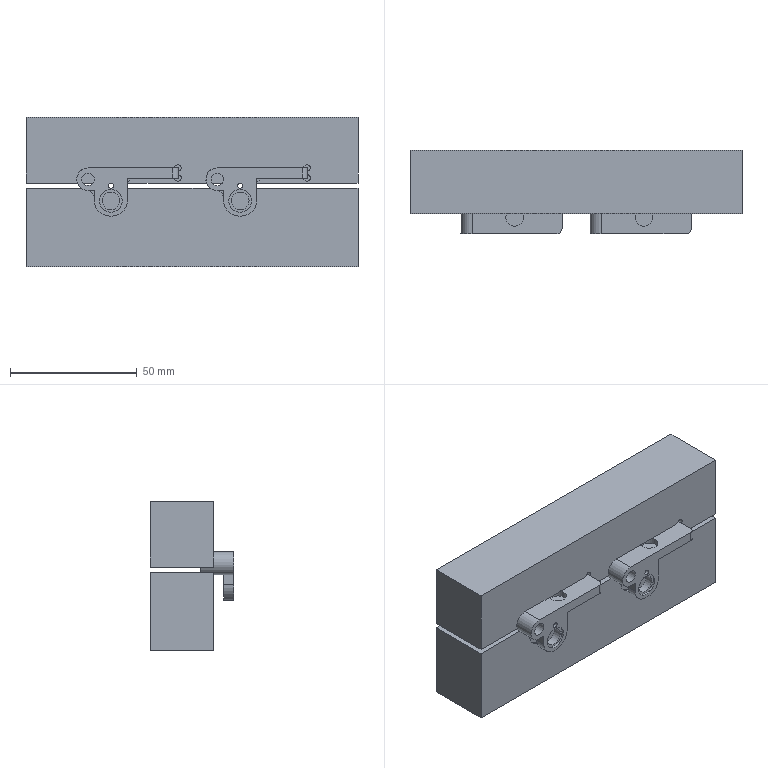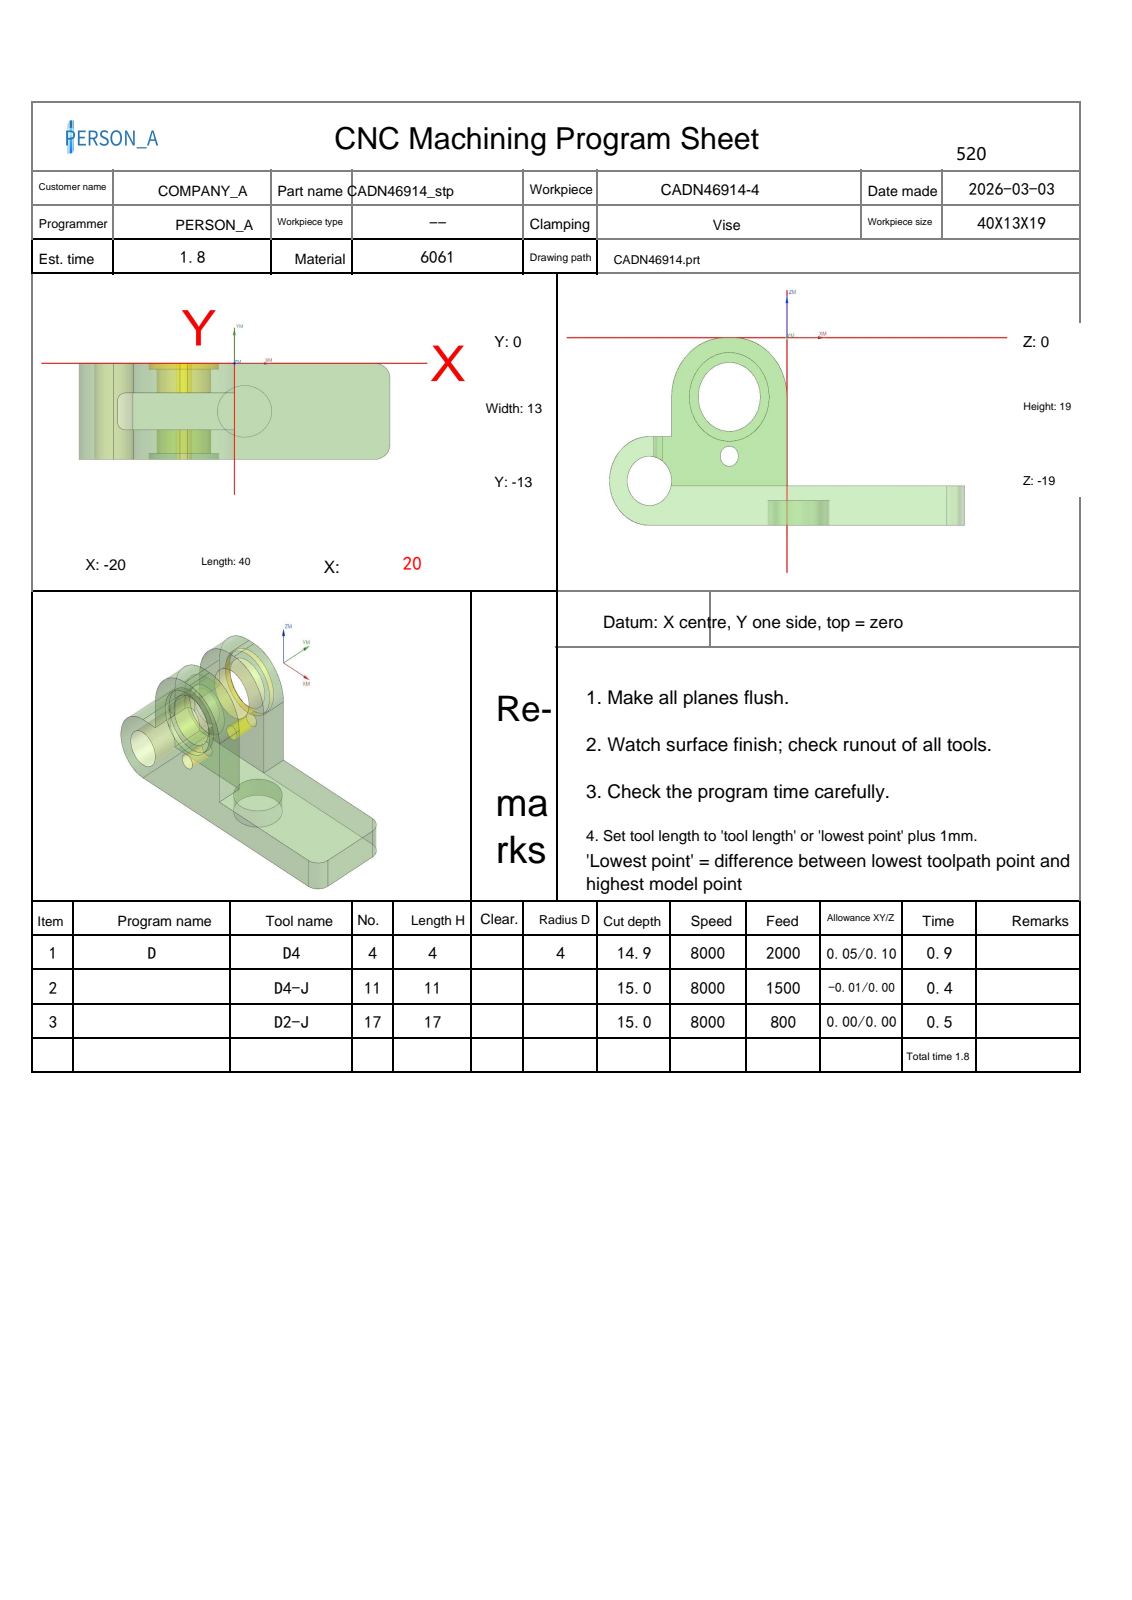NC program | NX | posted by the shop | part box 131 x 33 x 59 mm
Lines 1 to 812 of 3020:
%
O0001
(Machine time: 2.43 MIN)
(===Total Tool:3===)
(T4=D4      D=4.   R=0.   D4  H04 Z=-14.9 )
(T11=D4-J   D=4.   R=0.   D11 H11 Z=-15.  )
(T17=D2-J   D=2.   R=0.   D-  H17 Z=-15.  )
G80 G90 G17 G49 G40
G91 G28 Z0
M01
N1 T04 M06
(D4  D=4. R=0. H=04 ce=0.05 di=0.10)
G00 G90 G54 X2.6 Y-6.85 M03 S8000
G43 H04 Z10.334
M08
Z1.202
G01 Z-.298 F2000.
G41 D04
Y-6.65
G03 X2. Y-6.05 I-.6 J0.0
G01 X-12.95
Y-6.95
X2.
G03 X2.6 Y-6.35 I0.0 J.6
G01 G40 Y-6.15
Z1.202
G00 Z10.334
Y-6.85
Z.904
G01 Z-.596
G41 D04
Y-6.65
G03 X2. Y-6.05 I-.6 J0.0
G01 X-12.95
Y-6.95
X2.
G03 X2.6 Y-6.35 I0.0 J.6
G01 G40 Y-6.15
Z.904
G00 Z10.334
Y-6.85
Z.606
G01 Z-.894
G41 D04
Y-6.65
G03 X2. Y-6.05 I-.6 J0.0
G01 X-12.95
Y-6.95
X2.
G03 X2.6 Y-6.35 I0.0 J.6
G01 G40 Y-6.15
Z.606
G00 Z10.334
Y-6.85
Z.308
G01 Z-1.192
G41 D04
Y-6.65
G03 X2. Y-6.05 I-.6 J0.0
G01 X-12.95
Y-6.95
X2.
G03 X2.6 Y-6.35 I0.0 J.6
G01 G40 Y-6.15
Z.308
G00 Z10.334
Y-6.85
Z.01
G01 Z-1.49
G41 D04
Y-6.65
G03 X2. Y-6.05 I-.6 J0.0
G01 X-12.95
Y-6.95
X2.
G03 X2.6 Y-6.35 I0.0 J.6
G01 G40 Y-6.15
Z.01
G00 Y-6.85
Z-.288
G01 Z-1.788
G41 D04
Y-6.65
G03 X2. Y-6.05 I-.6 J0.0
G01 X-12.95
Y-6.95
X2.
G03 X2.6 Y-6.35 I0.0 J.6
G01 G40 Y-6.15
Z-.288
G00 Y-6.85
Z-.586
G01 Z-2.086
G41 D04
Y-6.65
G03 X2. Y-6.05 I-.6 J0.0
G01 X-12.95
Y-6.95
X2.
G03 X2.6 Y-6.35 I0.0 J.6
G01 G40 Y-6.15
Z-.586
G00 Y-6.85
Z-.884
G01 Z-2.384
G41 D04
Y-6.65
G03 X2. Y-6.05 I-.6 J0.0
G01 X-12.95
Y-6.95
X2.
G03 X2.6 Y-6.35 I0.0 J.6
G01 G40 Y-6.15
Z-.884
G00 Y-6.85
Z-1.182
G01 Z-2.682
G41 D04
Y-6.65
G03 X2. Y-6.05 I-.6 J0.0
G01 X-12.95
Y-6.95
X2.
G03 X2.6 Y-6.35 I0.0 J.6
G01 G40 Y-6.15
Z-1.182
G00 Y-6.85
Z-1.48
G01 Z-2.98
G41 D04
Y-6.65
G03 X2. Y-6.05 I-.6 J0.0
G01 X-12.95
Y-6.95
X2.
G03 X2.6 Y-6.35 I0.0 J.6
G01 G40 Y-6.15
Z-1.48
G00 Y-6.85
Z-1.778
G01 Z-3.278
G41 D04
Y-6.65
G03 X2. Y-6.05 I-.6 J0.0
G01 X-12.95
Y-6.95
X2.
G03 X2.6 Y-6.35 I0.0 J.6
G01 G40 Y-6.15
Z-1.778
G00 X2.333 Y-6.112
Z-2.076
G01 Z-3.576
G41 D04
X2.139 Y-6.066
X2.093 Y-6.054
X2.047 Y-6.049
X2. Y-6.05
X-12.95
Y-6.95
X2.
X2.047 Y-6.951
X2.093 Y-6.946
X2.139 Y-6.934
G40 X2.333 Y-6.888
Z-2.076
G00 X2.441 Y-6.197
Z-2.374
G01 Z-3.874
G41 D04
X2.261 Y-6.11
G03 X2. Y-6.05 I-.261 J-.54
G01 X-12.95
Y-6.95
X2.
G03 X2.261 Y-6.89 I0.0 J.6
G01 G40 X2.441 Y-6.803
Z-2.374
G00 X2.524 Y-6.295
Z-2.672
G01 Z-4.172
G41 D04
X2.365 Y-6.174
G03 X2. Y-6.05 I-.365 J-.476
G01 X-12.95
Y-6.95
X2.
G03 X2.365 Y-6.826 I0.0 J.6
G01 G40 X2.524 Y-6.705
Z-2.672
G00 X2.583 Y-6.406
Z-2.97
G01 Z-4.47
G41 D04
X2.452 Y-6.255
G03 X2. Y-6.05 I-.452 J-.395
G01 X-12.95
Y-6.95
X2.
G03 X2.452 Y-6.745 I0.0 J.6
G01 G40 X2.583 Y-6.594
Z-2.97
G00 X2.621 Y-6.528
Z-3.268
G01 Z-4.768
G41 D04
X2.522 Y-6.354
G03 X2. Y-6.05 I-.522 J-.296
G01 X-12.95
Y-6.95
X2.
G03 X2.522 Y-6.646 I0.0 J.6
G01 G40 X2.621 Y-6.472
Z-3.268
G00 X2.632 Y-6.677
Z-3.566
G01 Z-5.066
G41 D04
X2.577 Y-6.485
G03 X2. Y-6.05 I-.577 J-.165
G01 X-12.95
Y-6.95
X2.
G03 X2.577 Y-6.515 I0.0 J.6
G01 G40 X2.632 Y-6.323
Z-3.566
G00 X2.816 Y-6.65
Z-3.864
G01 Z-5.364
G41 D04
X2.6
G03 X2. Y-6.05 I-.6 J0.0
G01 X-12.95
Y-6.95
X2.
G03 X2.6 Y-6.35 I0.0 J.6
G01 X2.616
G40 X2.816
Z-3.864
G00 X2.84 Y-6.65
Z-4.162
G01 Z-5.662
G41 D04
X2.6
G03 X2. Y-6.05 I-.6 J0.0
G01 X-12.95
Y-6.95
X2.
G03 X2.6 Y-6.35 I0.0 J.6
G01 X2.64
G40 X2.84
Z-4.162
G00 X2.85 Y-6.65
Z-4.46
G01 Z-5.96
G41 D04
X2.6
G03 X2. Y-6.05 I-.6 J0.0
G01 X-12.95
Y-6.95
X2.
G03 X2.6 Y-6.35 I0.0 J.6
G01 X2.65
G40 X2.85
Z-4.46
G00 Y-6.65
Z-4.758
G01 Z-6.258
G41 D04
X2.6
G03 X2. Y-6.05 I-.6 J0.0
G01 X-12.95
Y-6.95
X2.
G03 X2.6 Y-6.35 I0.0 J.6
G01 X2.65
G40 X2.85
Z-4.758
G00 Y-6.65
Z-5.056
G01 Z-6.556
G41 D04
X2.6
G03 X2. Y-6.05 I-.6 J0.0
G01 X-12.95
Y-6.95
X2.
G03 X2.6 Y-6.35 I0.0 J.6
G01 X2.65
G40 X2.85
Z-5.056
G00 Y-6.65
Z-5.354
G01 Z-6.854
G41 D04
X2.6
G03 X2. Y-6.05 I-.6 J0.0
G01 X-12.95
Y-6.95
X2.
G03 X2.6 Y-6.35 I0.0 J.6
G01 X2.65
G40 X2.85
Z-5.354
G00 Y-6.65
Z-5.652
G01 Z-7.152
G41 D04
X2.6
G03 X2. Y-6.05 I-.6 J0.0
G01 X-12.95
Y-6.95
X2.
G03 X2.6 Y-6.35 I0.0 J.6
G01 X2.65
G40 X2.85
Z-5.652
G00 Y-6.65
Z-5.95
G01 Z-7.45
G41 D04
X2.6
G03 X2. Y-6.05 I-.6 J0.0
G01 X-12.95
Y-6.95
X2.
G03 X2.6 Y-6.35 I0.0 J.6
G01 X2.65
G40 X2.85
Z-5.95
G00 Y-6.65
Z-6.248
G01 Z-7.748
G41 D04
X2.6
G03 X2. Y-6.05 I-.6 J0.0
G01 X-12.95
Y-6.95
X2.
G03 X2.6 Y-6.35 I0.0 J.6
G01 X2.65
G40 X2.85
Z-6.248
G00 Y-6.65
Z-6.546
G01 Z-8.046
G41 D04
X2.6
G03 X2. Y-6.05 I-.6 J0.0
G01 X-12.95
Y-6.95
X2.
G03 X2.6 Y-6.35 I0.0 J.6
G01 X2.65
G40 X2.85
Z-6.546
G00 Y-6.65
Z-6.844
G01 Z-8.344
G41 D04
X2.6
G03 X2. Y-6.05 I-.6 J0.0
G01 X-12.95
Y-6.95
X2.
G03 X2.6 Y-6.35 I0.0 J.6
G01 X2.65
G40 X2.85
Z-6.844
G00 Y-6.65
Z-7.142
G01 Z-8.642
G41 D04
X2.6
G03 X2. Y-6.05 I-.6 J0.0
G01 X-12.95
Y-6.95
X2.
G03 X2.6 Y-6.35 I0.0 J.6
G01 X2.65
G40 X2.85
Z-7.142
G00 Y-6.65
Z-7.44
G01 Z-8.94
G41 D04
X2.6
G03 X2. Y-6.05 I-.6 J0.0
G01 X-12.95
Y-6.95
X2.
G03 X2.6 Y-6.35 I0.0 J.6
G01 X2.65
G40 X2.85
Z-7.44
G00 Y-6.65
Z-7.738
G01 Z-9.238
G41 D04
X2.6
G03 X2. Y-6.05 I-.6 J0.0
G01 X-12.95
Y-6.95
X2.
G03 X2.6 Y-6.35 I0.0 J.6
G01 X2.65
G40 X2.85
Z-7.738
G00 Y-6.65
Z-8.036
G01 Z-9.536
G41 D04
X2.6
G03 X2. Y-6.05 I-.6 J0.0
G01 X-12.95
Y-6.95
X2.
G03 X2.6 Y-6.35 I0.0 J.6
G01 X2.65
G40 X2.85
Z-8.036
G00 Y-6.65
Z-8.334
G01 Z-9.834
G41 D04
X2.6
G03 X2. Y-6.05 I-.6 J0.0
G01 X-12.95
Y-6.95
X2.
G03 X2.6 Y-6.35 I0.0 J.6
G01 X2.65
G40 X2.85
Z-8.334
G00 Y-6.65
Z-8.632
G01 Z-10.132
G41 D04
X2.6
G03 X2. Y-6.05 I-.6 J0.0
G01 X-12.95
Y-6.95
X2.
G03 X2.6 Y-6.35 I0.0 J.6
G01 X2.65
G40 X2.85
Z-8.632
G00 Y-6.65
Z-8.93
G01 Z-10.43
G41 D04
X2.6
G03 X2. Y-6.05 I-.6 J0.0
G01 X-12.95
Y-6.95
X2.
G03 X2.6 Y-6.35 I0.0 J.6
G01 X2.65
G40 X2.85
Z-8.93
G00 Y-6.65
Z-9.228
G01 Z-10.728
G41 D04
X2.6
G03 X2. Y-6.05 I-.6 J0.0
G01 X-12.95
Y-6.95
X2.
G03 X2.6 Y-6.35 I0.0 J.6
G01 X2.65
G40 X2.85
Z-9.228
G00 Y-6.65
Z-9.526
G01 Z-11.026
G41 D04
X2.6
G03 X2. Y-6.05 I-.6 J0.0
G01 X-12.95
Y-6.95
X2.
G03 X2.6 Y-6.35 I0.0 J.6
G01 X2.65
G40 X2.85
Z-9.526
G00 Y-6.65
Z-9.824
G01 Z-11.324
G41 D04
X2.6
G03 X2. Y-6.05 I-.6 J0.0
G01 X-12.95
Y-6.95
X2.
G03 X2.6 Y-6.35 I0.0 J.6
G01 X2.65
G40 X2.85
Z-9.824
G00 Y-6.65
Z-10.122
G01 Z-11.622
G41 D04
X2.6
G03 X2. Y-6.05 I-.6 J0.0
G01 X-12.95
Y-6.95
X2.
G03 X2.6 Y-6.35 I0.0 J.6
G01 X2.65
G40 X2.85
Z-10.122
G00 Y-6.65
Z-10.42
G01 Z-11.92
G41 D04
X2.6
G03 X2. Y-6.05 I-.6 J0.0
G01 X-12.95
Y-6.95
X2.
G03 X2.6 Y-6.35 I0.0 J.6
G01 X2.65
G40 X2.85
Z-10.42
G00 Y-6.65
Z-10.718
G01 Z-12.218
G41 D04
X2.6
G03 X2. Y-6.05 I-.6 J0.0
G01 X-12.95
Y-6.95
X2.
G03 X2.6 Y-6.35 I0.0 J.6
G01 X2.65
G40 X2.85
Z-10.718
G00 Y-6.65
Z-11.016
G01 Z-12.516
G41 D04
X2.6
G03 X2. Y-6.05 I-.6 J0.0
G01 X-12.95
Y-6.95
X2.
G03 X2.6 Y-6.35 I0.0 J.6
G01 X2.65
G40 X2.85
Z-11.016
G00 Y-6.65
Z-11.314
G01 Z-12.814
G41 D04
X2.6
G03 X2. Y-6.05 I-.6 J0.0
G01 X-12.95
Y-6.95
X2.
G03 X2.6 Y-6.35 I0.0 J.6
G01 X2.65
G40 X2.85
Z-11.314
G00 Y-6.65
Z-11.612
G01 Z-13.112
G41 D04
X2.6
G03 X2. Y-6.05 I-.6 J0.0
G01 X-12.95
Y-6.95
X2.
G03 X2.6 Y-6.35 I0.0 J.6
G01 X2.65
G40 X2.85
Z-11.612
G00 Y-6.65
Z-11.91
G01 Z-13.41
G41 D04
X2.6
G03 X2. Y-6.05 I-.6 J0.0
G01 X-12.95
Y-6.95
X2.
G03 X2.6 Y-6.35 I0.0 J.6
G01 X2.65
G40 X2.85
Z-11.91
G00 Y-6.65
Z-12.208
G01 Z-13.708
G41 D04
X2.6
G03 X2. Y-6.05 I-.6 J0.0
G01 X-12.95
Y-6.95
X2.
G03 X2.6 Y-6.35 I0.0 J.6
G01 X2.65
G40 X2.85
Z-12.208
G00 Y-6.65
Z-12.506
G01 Z-14.006
G41 D04
X2.6
G03 X2. Y-6.05 I-.6 J0.0
G01 X-12.95
Y-6.95
X2.
G03 X2.6 Y-6.35 I0.0 J.6
G01 X2.65
G40 X2.85
Z-12.506
G00 Y-6.65
Z-12.804
G01 Z-14.304
G41 D04
X2.6
G03 X2. Y-6.05 I-.6 J0.0
G01 X-12.95
Y-6.95
X2.
G03 X2.6 Y-6.35 I0.0 J.6
G01 X2.65
G40 X2.85
Z-12.804
G00 Y-6.65
Z-13.102
G01 Z-14.602
G41 D04
X2.6
G03 X2. Y-6.05 I-.6 J0.0
G01 X-12.95
Y-6.95
X2.
G03 X2.6 Y-6.35 I0.0 J.6
G01 X2.65
G40 X2.85
Z-13.102
G00 Y-6.65
Z-13.4
G01 Z-14.9
G41 D04
X2.6
G03 X2. Y-6.05 I-.6 J0.0
G01 X-12.95
Y-6.95
X2.
G03 X2.6 Y-6.35 I0.0 J.6
G01 X2.65
G40 X2.85
Z-13.4
G00 Z10.334
G91 G28 Z0.0
M05
M09
G91 G28 Z0.0
M01
N2 T11 M06
(D4-J  D=4. R=0. H=11 ce=0.40 di=0.00)
G00 G90 G54 X10.6 Y2.8 M03 S7000
G43 H11 Z10.4
M08
Z-13.5
G01 Z-15. F1500.
Y1.2
G03 X11.4 Y.4 I.8 J0.0
G01 X18.
G02 X20.4 Y-2. I0.0 J-2.4
G01 Y-11.
G02 X18. Y-13.4 I-2.4 J0.0
G01 X2.799
G02 X2.4 Y-13.001 I.001 J.4
G01 Y-6.6
X-12.52
X-12.565 Y-6.598
X-12.598 Y-6.565
X-12.6 Y-6.52
Y-6.48
X-12.598 Y-6.435
X-12.565 Y-6.402
X-12.52 Y-6.4
X2.4
Y.001
G02 X2.799 Y.4 I.4 J-.001
G01 X12.235
G02 X12.517 Y.283 I0.0 J-.4
G01 X14.283 Y-1.483
G03 X14.566 Y-1.6 I.283 J.283
G01 X18.
G02 X18.4 Y-2. I0.0 J-.4
G01 Y-11.
G02 X18. Y-11.4 I-.4 J0.0
G01 X4.799
G02 X4.4 Y-11.001 I.001 J.4
G01 Y-6.6
X4.397 Y-6.5
X4.4 Y-6.4
Y-1.999
G02 X4.799 Y-1.6 I.4 J-.001
G01 X12.235
G02 X12.517 Y-1.717 I0.0 J-.4
G01 X14.283 Y-3.483
G03 X14.566 Y-3.6 I.283 J.283
G01 X16.001
G02 X16.4 Y-3.999 I-.001 J-.4
G01 Y-9.001
G02 X16.001 Y-9.4 I-.4 J.001
G01 X6.799
G02 X6.4 Y-9.001 I.001 J.4
G01 Y-6.6
X6.399 Y-6.5
X6.4 Y-6.4
Y-3.999
G02 X6.799 Y-3.6 I.4 J-.001
G01 X12.208
G02 X12.52 Y-3.75 I0.0 J-.4
G01 X13.905 Y-5.48
G03 X14.109 Y-5.615 I.312 J.25
G02 X14.4 Y-5.999 I-.109 J-.385
G01 Y-7.001
G02 X14.001 Y-7.4 I-.4 J.001
G01 X8.799
G02 X8.4 Y-7.001 I.001 J.4
G01 Y-6.6
X8.399 Y-6.5
X8.4 Y-6.4
Y-5.999
G02 X8.799 Y-5.6 I.4 J-.001
G01 X13.4
X14.001
G02 X14.337 Y-5.784 I-.001 J-.4
G03 X15.01 Y-6.152 I.673 J.432
X15.442 Y-6.025 I0.0 J.8
G01 Z-13.5
G00 Z10.4
G00 G90 X-15.915 Y-15.817 M03 S8000
Z10.334
Z-4.
G01 Z-5. F800.
G41 D11
X-15.716 Y-15.796
G03 X-15. Y-15. I-.084 J.796
G01 Y2.
G03 X-15.716 Y2.796 I-.8 J0.0
G01 G40 X-15.915 Y2.817
Z-4.
G00 X-16. Y-15.8
Z-9.
G01 Z-10.
G41 D11
X-15.8
G03 X-15. Y-15. I0.0 J.8
G01 Y2.
G03 X-15.8 Y2.8 I-.8 J0.0
G01 G40 X-16.
Z-9.
G00 Z10.334
G00 G90 X2.861 Y2.822 M03 S8000
Z10.334
Z-4.
G01 Z-5. F800.
G41 D11
X2.664 Y2.79
G03 X1.99 Y2. I.126 J-.79
G01 Y-5.99
X-13.01
Y-7.01
X1.99
Y-15.
G03 X2.664 Y-15.79 I.8 J0.0
G01 G40 X2.861 Y-15.822
Z-4.
G00 Y2.822
Z-9.
G01 Z-10.
G41 D11
X2.664 Y2.79
G03 X1.99 Y2. I.126 J-.79
G01 Y-5.99
X-13.01
Y-7.01
X1.99
Y-15.
G03 X2.664 Y-15.79 I.8 J0.0
G01 G40 X2.861 Y-15.822
Z-9.
G00 Y2.822
Z-14.
G01 Z-15.
G41 D11
X2.664 Y2.79
G03 X1.99 Y2. I.126 J-.79
G01 Y-5.99
X-13.01
Y-7.01
X1.99
Y-15.
G03 X2.664 Y-15.79 I.8 J0.0
G01 G40 X2.861 Y-15.822
Z-14.
G00 Z10.334
G91 G28 Z0.0
M05
M09
G91 G28 Z0.0
M01